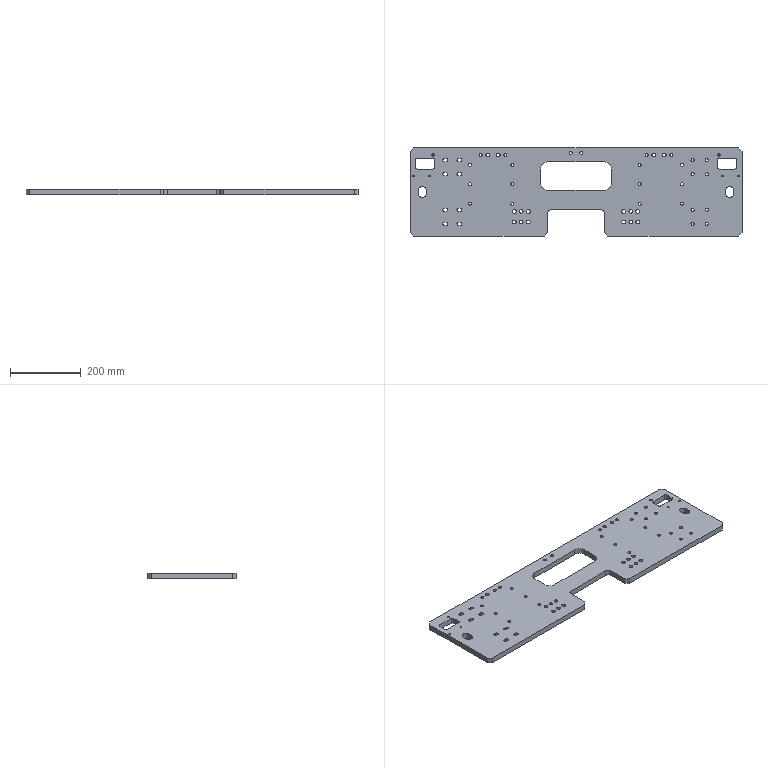Part | SolidWorks | features BaseBody 1 | 1 solid | 186 faces | box 940 x 250 x 16 mm | volume 3179038 mm3 | cylinder 138 | plane 48 | commonest cylinder face diameters 9 x40 8.5 x36 10 x24 11 x16 5 x8 6.8 x4